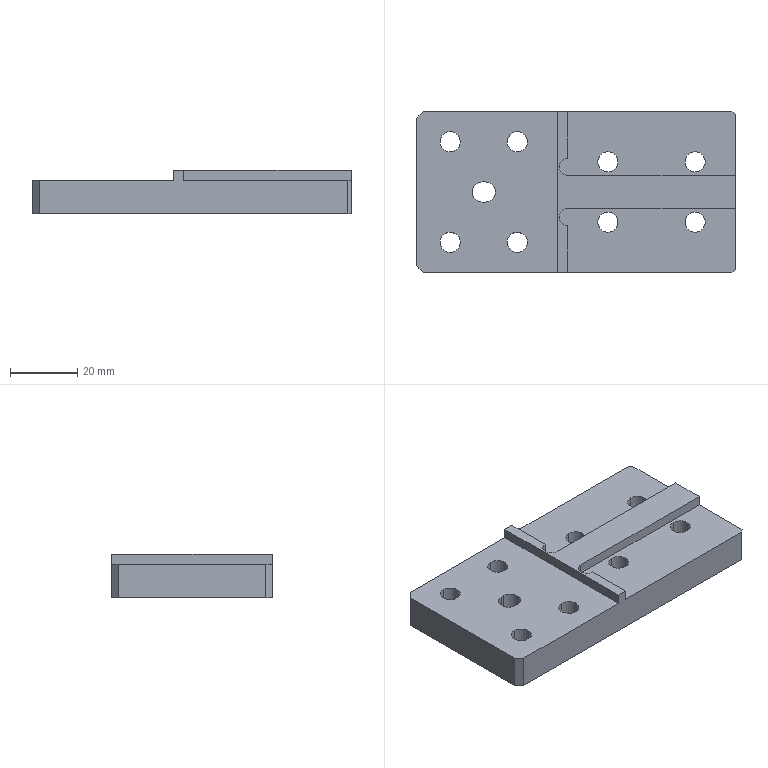Part | STEP file | J454-EBZ05-36-04-Part-2-4 | 1 solid | 40 faces | box 95 x 48 x 13 mm | volume 44818 mm3 | cylinder 20 | plane 20 | commonest cylinder face diameters 6 x18 5 x2